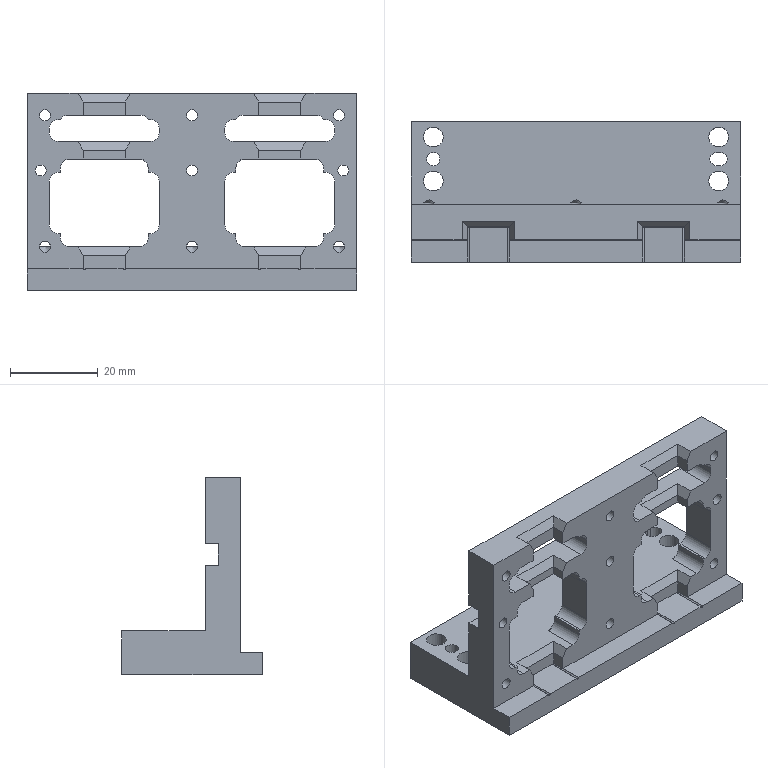CAM job | NX | 3+2 milling, drilling | part box 75 x 32 x 45 mm | stock box 80 x 35 x 50 mm
Tools:
number,name,description,diameter,corner_radius,flute_length,length,flutes
4,D4,平底铣刀-粗,4.0,0.0,25.0,75.0,2
6,D6,平底铣刀-粗,6.0,0.0,25.0,75.0,2
9,D10,平底铣刀-粗,10.0,0.0,35.0,75.0,2
19,D2-J,平底铣刀-精,2.0,0.0,50.0,75.0,2
11,D4-J,平底铣刀-精,4.0,0.0,50.0,75.0,2
7,D6-J,平底铣刀-精,6.0,0.0,25.0,75.0,2
10,D10-J,平底铣刀-精,10.0,0.0,35.0,75.0,2
2,D6倒角刀,倒角刀,6.0,0.0,3.0,25.0,2
18,D3铰刀,Drilling Tool,3.0,0.0,75.0,100.0,6
17,ZT3.1,钻头,3.1,0.0,35.0,50.0,2
11,ZT4.5,钻头,4.5,0.0,35.0,50.0,2
17,ZT2.9,Drilling Tool,2.9,0.0,35.0,50.0,2
Operations:
program,operation,operation_type,tool,method,geometry_group,spindle_rpm,surface_speed,feed_per_tooth,feed_cut,feed_plunge,cut_length_mm,path_length_mm,cut_time_min,machine_time_min
C,打点-深0.8_2,Operation,D6倒角刀,NONE,W-C,8000.0,150.796,0.0312,500.0,90.0,9.0,167.256,0.018,0.0338
C,打点-深0.8_2_COPY,Operation,D6倒角刀,NONE,W-C,8000.0,150.796,0.0312,500.0,90.0,1.8,63.6,0.0036,0.0098
C,通孔-精孔3.0预钻,Operation,ZT2.9,NONE,W-C,3200.0,29.154,0.0312,200.0,90.0,14.837,89.674,0.0742,0.0817
C,通孔-精孔3.0预钻_COPY,Operation,ZT2.9,NONE,W-C,3200.0,29.154,0.0312,200.0,90.0,14.837,89.674,0.0742,0.0817
C,通孔-5-6,Operation,ZT4.5,NONE,W-C,3000.0,42.411,0.025,150.0,90.0,57.408,262.923,0.3827,0.4033
C,底壁铣螺旋开粗-小_COPY,VolumeBased25DMillingOperation,D2-J,分层开粗-切深K-步距G,W-C,8000.0,50.264,0.0375,600.0,100.0,526.407,595.307,0.8773,0.8842
C,钻倒角_2,Operation,D6倒角刀,METHOD,W-C,8000.0,150.796,0.0312,500.0,0.0,4.8,69.6,0.0096,0.0161
C,铣倒角_1,PlanarMilling,D6倒角刀,METHOD,W-C,8000.0,150.796,0.0312,500.0,100.0,69.412,398.421,0.1388,0.1717
C,C0.3封闭铣廓倒角6X45L_COPY,PlanarMilling,D6倒角刀,爬面_倒角-切深0-步距G,W-C,7000.0,131.0,0.1071,1500.0,100.0,19.317,75.317,0.0129,0.0185
C,REAMING,Operation,D3铰刀,METHOD,W-C,500.0,4.712,0.0167,50.0,0.0,12.0,84.0,0.24,0.2472
C,底壁铣螺旋精光-小_COPY,VolumeBased25DMillingOperation,D2-J,螺旋精光-切深K-步距G,W-C,8000.0,50.266,0.0125,200.0,100.0,74.574,143.574,0.3729,0.3798
B,面铣自动飞面开粗_COPY,FaceMilling,D6,分层开粗-切深K-步距G,W-B,8000.0,150.796,0.25,4000.0,100.0,9534.328,9917.957,2.384,2.422
B,底壁铣分层开粗-中_COPY_1,VolumeBased25DMillingOperation,D6,分层开粗-切深K-步距G,W-B,8000.0,150.796,0.25,4000.0,100.0,29194.311,32702.059,7.299,7.649
B,面铣自动飞面精光_COPY,FaceMilling,D6-J,侧刃精光-切深K-步距G,W-B,8000.0,150.796,0.0625,1000.0,100.0,1043.154,1139.154,1.043,1.053
B,底壁铣分层开粗-中_COPY_2,VolumeBased25DMillingOperation,D4,分层开粗-切深K-步距G,W-B,8000.0,100.528,0.125,2000.0,100.0,1517.351,1650.757,0.7587,0.772
B,平面去毛刺6X45L_COPY,SurfaceContour,D6倒角刀,爬面_倒角-切深0-步距G,W-B,6500.0,122.519,0.1154,1500.0,100.0,723.979,1632.407,0.4827,0.5735
B,底壁铣精光侧面-中-选底面_COPY,VolumeBased25DMillingOperation,D4-J,侧刃精光-切深K-步距G,W-B,8000.0,100.528,0.05,800.0,100.0,115.962,346.418,0.145,0.168
B,底壁铣精光底面-中_COPY_2,VolumeBased25DMillingOperation,D6-J,精光步距切深关,W-B,7000.0,175.0,0.0536,1500.0,100.0,742.138,802.138,0.4948,0.5008
B,等高精光-中_COPY_2,ZLevelMilling,D6-J,侧刃精光-切深K-步距G,W-B,8000.0,150.792,0.0625,1000.0,100.0,320.077,587.77,0.3201,0.3468
A,顶面,FaceMilling,D10-J,侧刃精光-切深K-步距G,W-A,4500.0,1385.0,0.1667,1500.0,100.0,650.25,706.25,0.4335,0.4391
A,外形粗_2,VolumeBased25DMillingOperation,D10,METHOD,W-A,8000.0,251.327,0.375,6000.0,80.0,11427.406,11517.906,1.905,1.914
A,底壁铣分层开粗-中_COPY,VolumeBased25DMillingOperation,D6,分层开粗-切深K-步距G,W-A,8000.0,150.792,0.1875,3000.0,100.0,8618.555,8804.607,2.873,2.892
A,型腔铣开粗-中_COPY,CavityMilling,D4,分层开粗-切深K-步距G,W-A,8000.0,100.531,0.125,2000.0,100.0,11649.437,12871.507,5.825,5.99
A,打点-深0.8,Operation,D6倒角刀,NONE,W-A,8000.0,150.796,0.0312,500.0,90.0,16.2,267.771,0.0324,0.0576
A,通孔-M3螺纹底孔,Operation,ZT3.1,NONE,W-A,3000.0,23.562,0.05,300.0,90.0,66.0,313.027,0.22,0.2447
A,盲锥孔-M3螺纹底孔,Operation,ZT3.1,NONE,W-A,3000.0,23.562,0.0167,100.0,90.0,31.5,202.03,0.315,0.3321
A,仅选体,SurfaceContour,D6倒角刀,METHOD,W-A,8000.0,150.796,0.1875,3000.0,100.0,671.335,1262.974,0.2238,0.2829
A,钻倒角_1,Operation,D6倒角刀,METHOD,W-A,8000.0,150.796,0.0312,500.0,0.0,42.75,338.729,0.0855,0.1151
A,外形半精_2,VolumeBased25DMillingOperation,D10-J,METHOD,W-A,9000.0,169.646,0.0667,1200.0,100.0,829.122,1139.151,0.6909,0.7219
A,底壁铣精光底面-中_COPY,VolumeBased25DMillingOperation,D4-J,精光步距切深关,W-A,7000.0,175.0,0.0536,1500.0,100.0,992.124,1116.789,0.6614,0.6739
A,等高精光-中_COPY,ZLevelMilling,D4-J,侧刃精光-切深K-步距G,W-A,8000.0,100.528,0.05,800.0,100.0,1003.516,1882.709,1.254,1.342
A,底壁铣精光底面-中_COPY_1,VolumeBased25DMillingOperation,D4-J,精光步距切深关,W-A,7000.0,175.0,0.0536,1500.0,100.0,140.192,246.702,0.0935,0.1041
A,等高精光-中_COPY_1,ZLevelMilling,D4-J,侧刃精光-切深K-步距G,W-A,8000.0,100.528,0.05,800.0,100.0,79.151,98.151,0.0989,0.1008
A,等高精光往复爬面_COPY,ZLevelMilling,D4-J,等高爬面-切深K-步距G,W-A,8000.0,100.531,0.1875,3000.0,100.0,7972.861,8375.179,2.658,2.698
A,等高光顺清角D2参考6_COPY,ZLevelMilling,D2-J,分层精光-切深K-步距G,W-A,8000.0,50.264,0.05,800.0,100.0,1336.647,1699.473,1.671,1.707